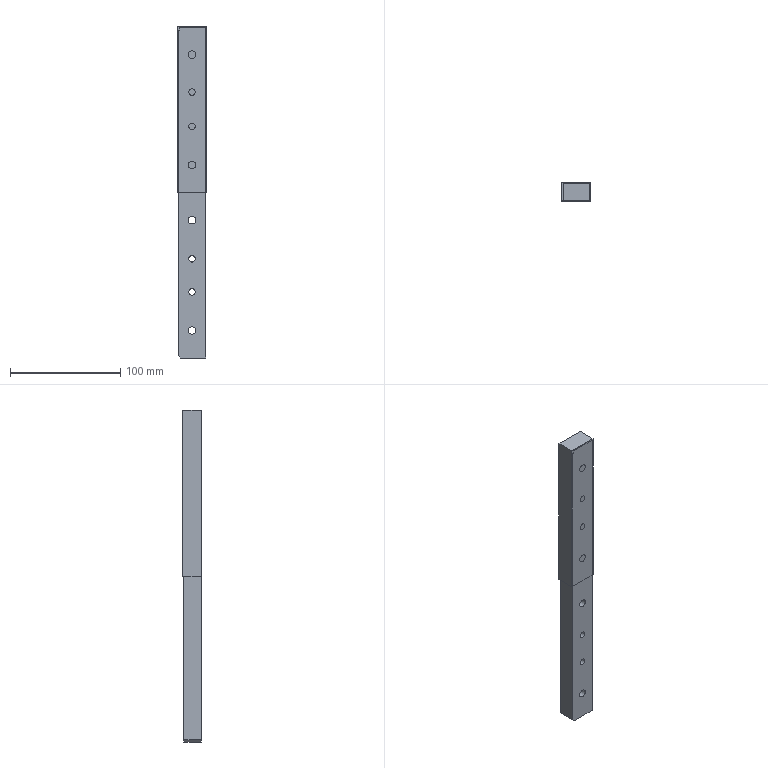Part | NX | features BREP 2 | 2 solids | 39 faces | box 27 x 16.6 x 301 mm | volume 178522 mm3 | plane 23 | cylinder 16 | commonest cylinder face diameters 7 x8 6 x4 11 x4
STEP:
#1=CARTESIAN_POINT('',(12.5,15.6,280.5));
#2=VERTEX_POINT('',#1);
#3=CARTESIAN_POINT('',(12.5,15.6,275.));
#4=DIRECTION('',(0.,1.,0.));
#5=DIRECTION('',(0.,0.,1.));
#6=AXIS2_PLACEMENT_3D('',#3,#4,#5);
#7=CIRCLE('',#6,5.5);
#8=EDGE_CURVE('',#2,#2,#7,.T.);
#9=ORIENTED_EDGE('',*,*,#8,.F.);
#10=EDGE_LOOP('',(#9));
#11=FACE_BOUND('',#10,.T.);
#12=CARTESIAN_POINT('',(12.5,15.6,213.5));
#13=VERTEX_POINT('',#12);
#14=CARTESIAN_POINT('',(12.5,15.6,210.));
#15=DIRECTION('',(0.,1.,0.));
#16=DIRECTION('',(0.,0.,1.));
#17=AXIS2_PLACEMENT_3D('',#14,#15,#16);
#18=CIRCLE('',#17,3.5);
#19=EDGE_CURVE('',#13,#13,#18,.T.);
#20=ORIENTED_EDGE('',*,*,#19,.F.);
#21=EDGE_LOOP('',(#20));
#22=FACE_BOUND('',#21,.T.);
#23=CARTESIAN_POINT('',(12.5,15.6,244.5));
#24=VERTEX_POINT('',#23);
#25=CARTESIAN_POINT('',(12.5,15.6,241.));
#26=DIRECTION('',(0.,1.,0.));
#27=DIRECTION('',(0.,0.,1.));
#28=AXIS2_PLACEMENT_3D('',#25,#26,#27);
#29=CIRCLE('',#28,3.5);
#30=EDGE_CURVE('',#24,#24,#29,.T.);
#31=ORIENTED_EDGE('',*,*,#30,.F.);
#32=EDGE_LOOP('',(#31));
#33=FACE_BOUND('',#32,.T.);
#34=CARTESIAN_POINT('',(12.5,15.6,180.5));
#35=VERTEX_POINT('',#34);
#36=CARTESIAN_POINT('',(12.5,15.6,175.));
#37=DIRECTION('',(0.,1.,0.));
#38=DIRECTION('',(0.,0.,1.));
#39=AXIS2_PLACEMENT_3D('',#36,#37,#38);
#40=CIRCLE('',#39,5.5);
#41=EDGE_CURVE('',#35,#35,#40,.T.);
#42=ORIENTED_EDGE('',*,*,#41,.F.);
#43=EDGE_LOOP('',(#42));
#44=FACE_BOUND('',#43,.T.);
#45=CARTESIAN_POINT('',(12.5,15.6,63.5));
#46=VERTEX_POINT('',#45);
#47=CARTESIAN_POINT('',(12.5,15.6,60.));
#48=DIRECTION('',(0.,1.,0.));
#49=DIRECTION('',(0.,0.,1.));
#50=AXIS2_PLACEMENT_3D('',#47,#48,#49);
#51=CIRCLE('',#50,3.5);
#52=EDGE_CURVE('',#46,#46,#51,.T.);
#53=ORIENTED_EDGE('',*,*,#52,.F.);
#54=EDGE_LOOP('',(#53));
#55=FACE_BOUND('',#54,.T.);
#56=CARTESIAN_POINT('',(12.5,15.6,93.5));
#57=VERTEX_POINT('',#56);
#58=CARTESIAN_POINT('',(12.5,15.6,90.));
#59=DIRECTION('',(0.,1.,0.));
#60=DIRECTION('',(0.,0.,1.));
#61=AXIS2_PLACEMENT_3D('',#58,#59,#60);
#62=CIRCLE('',#61,3.5);
#63=EDGE_CURVE('',#57,#57,#62,.T.);
#64=ORIENTED_EDGE('',*,*,#63,.F.);
#65=EDGE_LOOP('',(#64));
#66=FACE_BOUND('',#65,.T.);
#67=CARTESIAN_POINT('',(12.5,15.6,30.5));
#68=VERTEX_POINT('',#67);
#69=CARTESIAN_POINT('',(12.5,15.6,25.));
#70=DIRECTION('',(0.,1.,0.));
#71=DIRECTION('',(0.,0.,1.));
#72=AXIS2_PLACEMENT_3D('',#69,#70,#71);
#73=CIRCLE('',#72,5.5);
#74=EDGE_CURVE('',#68,#68,#73,.T.);
#75=ORIENTED_EDGE('',*,*,#74,.F.);
#76=EDGE_LOOP('',(#75));
#77=FACE_BOUND('',#76,.T.);
#78=CARTESIAN_POINT('',(12.5,15.6,130.5));
#79=VERTEX_POINT('',#78);
#80=CARTESIAN_POINT('',(12.5,15.6,125.));
#81=DIRECTION('',(0.,1.,0.));
#82=DIRECTION('',(0.,0.,1.));
#83=AXIS2_PLACEMENT_3D('',#80,#81,#82);
#84=CIRCLE('',#83,5.5);
#85=EDGE_CURVE('',#79,#79,#84,.T.);
#86=ORIENTED_EDGE('',*,*,#85,.F.);
#87=EDGE_LOOP('',(#86));
#88=FACE_BOUND('',#87,.T.);
#89=CARTESIAN_POINT('',(0.,15.6,297.342));
#90=VERTEX_POINT('',#89);
#91=CARTESIAN_POINT('',(0.,15.6,2.));
#92=VERTEX_POINT('',#91);
#93=CARTESIAN_POINT('',(0.,15.6,300.));
#94=DIRECTION('',(0.,0.,-1.));
#95=VECTOR('',#94,1000.);
#96=LINE('',#93,#95);
#97=EDGE_CURVE('',#90,#92,#96,.T.);
#98=ORIENTED_EDGE('',*,*,#97,.F.);
#99=CARTESIAN_POINT('',(0.9,15.6,297.342));
#100=VERTEX_POINT('',#99);
#101=CARTESIAN_POINT('',(0.,15.6,297.342));
#102=DIRECTION('',(1.,0.,0.));
#103=VECTOR('',#102,1000.);
#104=LINE('',#101,#103);
#105=EDGE_CURVE('',#90,#100,#104,.T.);
#106=ORIENTED_EDGE('',*,*,#105,.T.);
#107=CARTESIAN_POINT('',(0.9,15.6,300.));
#108=VERTEX_POINT('',#107);
#109=CARTESIAN_POINT('',(0.9,15.6,300.));
#110=DIRECTION('',(0.,0.,1.));
#111=VECTOR('',#110,1000.);
#112=LINE('',#109,#111);
#113=EDGE_CURVE('',#100,#108,#112,.T.);
#114=ORIENTED_EDGE('',*,*,#113,.T.);
#115=CARTESIAN_POINT('',(25.,15.6,300.));
#116=VERTEX_POINT('',#115);
#117=CARTESIAN_POINT('',(0.,15.6,300.));
#118=DIRECTION('',(1.,0.,0.));
#119=VECTOR('',#118,1000.);
#120=LINE('',#117,#119);
#121=EDGE_CURVE('',#108,#116,#120,.T.);
#122=ORIENTED_EDGE('',*,*,#121,.T.);
#123=CARTESIAN_POINT('',(25.,15.6,0.));
#124=VERTEX_POINT('',#123);
#125=CARTESIAN_POINT('',(25.,15.6,300.));
#126=DIRECTION('',(0.,0.,-1.));
#127=VECTOR('',#126,1000.);
#128=LINE('',#125,#127);
#129=EDGE_CURVE('',#116,#124,#128,.T.);
#130=ORIENTED_EDGE('',*,*,#129,.T.);
#131=CARTESIAN_POINT('',(2.,15.6,0.));
#132=VERTEX_POINT('',#131);
#133=CARTESIAN_POINT('',(0.,15.6,0.));
#134=DIRECTION('',(1.,0.,0.));
#135=VECTOR('',#134,1000.);
#136=LINE('',#133,#135);
#137=EDGE_CURVE('',#132,#124,#136,.T.);
#138=ORIENTED_EDGE('',*,*,#137,.F.);
#139=CARTESIAN_POINT('',(-149.,15.6,151.));
#140=DIRECTION('',(-0.7071,0.,0.7071));
#141=VECTOR('',#140,1000.);
#142=LINE('',#139,#141);
#143=EDGE_CURVE('',#132,#92,#142,.T.);
#144=ORIENTED_EDGE('',*,*,#143,.T.);
#145=EDGE_LOOP('',(#98,#106,#114,#122,#130,#138,#144));
#146=FACE_BOUND('',#145,.T.);
#147=CARTESIAN_POINT('',(0.,15.6,300.));
#148=DIRECTION('',(0.,1.,0.));
#149=DIRECTION('',(0.,0.,-1.));
#150=AXIS2_PLACEMENT_3D('',#147,#148,#149);
#151=PLANE('',#150);
#152=ADVANCED_FACE('',(#11,#22,#33,#44,#55,#66,#77,#88,#146),#151,.T.);
#153=CARTESIAN_POINT('',(0.,0.,297.342));
#154=VERTEX_POINT('',#153);
#155=CARTESIAN_POINT('',(0.,0.,2.));
#156=VERTEX_POINT('',#155);
#157=CARTESIAN_POINT('',(0.,0.,300.));
#158=DIRECTION('',(0.,0.,-1.));
#159=VECTOR('',#158,1000.);
#160=LINE('',#157,#159);
#161=EDGE_CURVE('',#154,#156,#160,.T.);
#162=ORIENTED_EDGE('',*,*,#161,.F.);
#163=CARTESIAN_POINT('',(0.,0.,297.342));
#164=DIRECTION('',(0.,1.,0.));
#165=VECTOR('',#164,1000.);
#166=LINE('',#163,#165);
#167=EDGE_CURVE('',#154,#90,#166,.T.);
#168=ORIENTED_EDGE('',*,*,#167,.T.);
#169=ORIENTED_EDGE('',*,*,#97,.T.);
#170=CARTESIAN_POINT('',(0.,0.,2.));
#171=DIRECTION('',(0.,-1.,0.));
#172=VECTOR('',#171,1000.);
#173=LINE('',#170,#172);
#174=EDGE_CURVE('',#92,#156,#173,.T.);
#175=ORIENTED_EDGE('',*,*,#174,.T.);
#176=EDGE_LOOP('',(#162,#168,#169,#175));
#177=FACE_BOUND('',#176,.T.);
#178=CARTESIAN_POINT('',(0.,0.,300.));
#179=DIRECTION('',(-1.,0.,0.));
#180=DIRECTION('',(0.,0.,-1.));
#181=AXIS2_PLACEMENT_3D('',#178,#179,#180);
#182=PLANE('',#181);
#183=ADVANCED_FACE('',(#177),#182,.T.);
#184=CARTESIAN_POINT('',(12.5,0.,271.5));
#185=VERTEX_POINT('',#184);
#186=CARTESIAN_POINT('',(12.5,0.,275.));
#187=DIRECTION('',(0.,-1.,0.));
#188=DIRECTION('',(0.,0.,-1.));
#189=AXIS2_PLACEMENT_3D('',#186,#187,#188);
#190=CIRCLE('',#189,3.5);
#191=EDGE_CURVE('',#185,#185,#190,.T.);
#192=ORIENTED_EDGE('',*,*,#191,.F.);
#193=EDGE_LOOP('',(#192));
#194=FACE_BOUND('',#193,.T.);
#195=CARTESIAN_POINT('',(15.5,0.,210.));
#196=VERTEX_POINT('',#195);
#197=CARTESIAN_POINT('',(12.5,0.,210.));
#198=DIRECTION('',(0.,-1.,0.));
#199=DIRECTION('',(1.,0.,0.));
#200=AXIS2_PLACEMENT_3D('',#197,#198,#199);
#201=CIRCLE('',#200,3.);
#202=EDGE_CURVE('',#196,#196,#201,.T.);
#203=ORIENTED_EDGE('',*,*,#202,.F.);
#204=EDGE_LOOP('',(#203));
#205=FACE_BOUND('',#204,.T.);
#206=CARTESIAN_POINT('',(15.5,0.,241.));
#207=VERTEX_POINT('',#206);
#208=CARTESIAN_POINT('',(12.5,0.,241.));
#209=DIRECTION('',(0.,-1.,0.));
#210=DIRECTION('',(1.,0.,0.));
#211=AXIS2_PLACEMENT_3D('',#208,#209,#210);
#212=CIRCLE('',#211,3.);
#213=EDGE_CURVE('',#207,#207,#212,.T.);
#214=ORIENTED_EDGE('',*,*,#213,.F.);
#215=EDGE_LOOP('',(#214));
#216=FACE_BOUND('',#215,.T.);
#217=CARTESIAN_POINT('',(12.5,0.,171.5));
#218=VERTEX_POINT('',#217);
#219=CARTESIAN_POINT('',(12.5,0.,175.));
#220=DIRECTION('',(0.,-1.,0.));
#221=DIRECTION('',(0.,0.,-1.));
#222=AXIS2_PLACEMENT_3D('',#219,#220,#221);
#223=CIRCLE('',#222,3.5);
#224=EDGE_CURVE('',#218,#218,#223,.T.);
#225=ORIENTED_EDGE('',*,*,#224,.F.);
#226=EDGE_LOOP('',(#225));
#227=FACE_BOUND('',#226,.T.);
#228=CARTESIAN_POINT('',(15.5,0.,60.));
#229=VERTEX_POINT('',#228);
#230=CARTESIAN_POINT('',(12.5,0.,60.));
#231=DIRECTION('',(0.,-1.,0.));
#232=DIRECTION('',(1.,0.,0.));
#233=AXIS2_PLACEMENT_3D('',#230,#231,#232);
#234=CIRCLE('',#233,3.);
#235=EDGE_CURVE('',#229,#229,#234,.T.);
#236=ORIENTED_EDGE('',*,*,#235,.F.);
#237=EDGE_LOOP('',(#236));
#238=FACE_BOUND('',#237,.T.);
#239=CARTESIAN_POINT('',(15.5,0.,90.));
#240=VERTEX_POINT('',#239);
#241=CARTESIAN_POINT('',(12.5,0.,90.));
#242=DIRECTION('',(0.,-1.,0.));
#243=DIRECTION('',(1.,0.,0.));
#244=AXIS2_PLACEMENT_3D('',#241,#242,#243);
#245=CIRCLE('',#244,3.);
#246=EDGE_CURVE('',#240,#240,#245,.T.);
#247=ORIENTED_EDGE('',*,*,#246,.F.);
#248=EDGE_LOOP('',(#247));
#249=FACE_BOUND('',#248,.T.);
#250=CARTESIAN_POINT('',(12.5,0.,21.5));
#251=VERTEX_POINT('',#250);
#252=CARTESIAN_POINT('',(12.5,0.,25.));
#253=DIRECTION('',(0.,-1.,0.));
#254=DIRECTION('',(0.,0.,-1.));
#255=AXIS2_PLACEMENT_3D('',#252,#253,#254);
#256=CIRCLE('',#255,3.5);
#257=EDGE_CURVE('',#251,#251,#256,.T.);
#258=ORIENTED_EDGE('',*,*,#257,.F.);
#259=EDGE_LOOP('',(#258));
#260=FACE_BOUND('',#259,.T.);
#261=CARTESIAN_POINT('',(12.5,0.,121.5));
#262=VERTEX_POINT('',#261);
#263=CARTESIAN_POINT('',(12.5,0.,125.));
#264=DIRECTION('',(0.,-1.,0.));
#265=DIRECTION('',(0.,0.,-1.));
#266=AXIS2_PLACEMENT_3D('',#263,#264,#265);
#267=CIRCLE('',#266,3.5);
#268=EDGE_CURVE('',#262,#262,#267,.T.);
#269=ORIENTED_EDGE('',*,*,#268,.F.);
#270=EDGE_LOOP('',(#269));
#271=FACE_BOUND('',#270,.T.);
#272=CARTESIAN_POINT('',(0.9,0.,300.));
#273=VERTEX_POINT('',#272);
#274=CARTESIAN_POINT('',(0.9,0.,297.342));
#275=VERTEX_POINT('',#274);
#276=CARTESIAN_POINT('',(0.9,0.,300.));
#277=DIRECTION('',(0.,0.,-1.));
#278=VECTOR('',#277,1000.);
#279=LINE('',#276,#278);
#280=EDGE_CURVE('',#273,#275,#279,.T.);
#281=ORIENTED_EDGE('',*,*,#280,.T.);
#282=CARTESIAN_POINT('',(25.,0.,297.342));
#283=DIRECTION('',(-1.,0.,0.));
#284=VECTOR('',#283,1000.);
#285=LINE('',#282,#284);
#286=EDGE_CURVE('',#275,#154,#285,.T.);
#287=ORIENTED_EDGE('',*,*,#286,.T.);
#288=ORIENTED_EDGE('',*,*,#161,.T.);
#289=CARTESIAN_POINT('',(2.,0.,0.));
#290=VERTEX_POINT('',#289);
#291=CARTESIAN_POINT('',(-136.5,0.,138.5));
#292=DIRECTION('',(0.7071,0.,-0.7071));
#293=VECTOR('',#292,1000.);
#294=LINE('',#291,#293);
#295=EDGE_CURVE('',#156,#290,#294,.T.);
#296=ORIENTED_EDGE('',*,*,#295,.T.);
#297=CARTESIAN_POINT('',(25.,0.,0.));
#298=VERTEX_POINT('',#297);
#299=CARTESIAN_POINT('',(25.,0.,0.));
#300=DIRECTION('',(-1.,0.,0.));
#301=VECTOR('',#300,1000.);
#302=LINE('',#299,#301);
#303=EDGE_CURVE('',#298,#290,#302,.T.);
#304=ORIENTED_EDGE('',*,*,#303,.F.);
#305=CARTESIAN_POINT('',(25.,0.,300.));
#306=VERTEX_POINT('',#305);
#307=CARTESIAN_POINT('',(25.,0.,300.));
#308=DIRECTION('',(0.,0.,-1.));
#309=VECTOR('',#308,1000.);
#310=LINE('',#307,#309);
#311=EDGE_CURVE('',#306,#298,#310,.T.);
#312=ORIENTED_EDGE('',*,*,#311,.F.);
#313=CARTESIAN_POINT('',(25.,0.,300.));
#314=DIRECTION('',(-1.,0.,0.));
#315=VECTOR('',#314,1000.);
#316=LINE('',#313,#315);
#317=EDGE_CURVE('',#306,#273,#316,.T.);
#318=ORIENTED_EDGE('',*,*,#317,.T.);
#319=EDGE_LOOP('',(#281,#287,#288,#296,#304,#312,#318));
#320=FACE_BOUND('',#319,.T.);
#321=CARTESIAN_POINT('',(25.,0.,300.));
#322=DIRECTION('',(0.,-1.,0.));
#323=DIRECTION('',(-1.,0.,0.));
#324=AXIS2_PLACEMENT_3D('',#321,#322,#323);
#325=PLANE('',#324);
#326=ADVANCED_FACE('',(#194,#205,#216,#227,#238,#249,#260,#271,#320),#325,.T.);
#327=CARTESIAN_POINT('',(0.9,0.,300.));
#328=DIRECTION('',(0.,1.,0.));
#329=VECTOR('',#328,1000.);
#330=LINE('',#327,#329);
#331=EDGE_CURVE('',#273,#108,#330,.T.);
#332=ORIENTED_EDGE('',*,*,#331,.F.);
#333=ORIENTED_EDGE('',*,*,#317,.F.);
#334=CARTESIAN_POINT('',(25.,15.6,300.));
#335=DIRECTION('',(0.,-1.,0.));
#336=VECTOR('',#335,1000.);
#337=LINE('',#334,#336);
#338=EDGE_CURVE('',#116,#306,#337,.T.);
#339=ORIENTED_EDGE('',*,*,#338,.F.);
#340=ORIENTED_EDGE('',*,*,#121,.F.);
#341=EDGE_LOOP('',(#332,#333,#339,#340));
#342=FACE_BOUND('',#341,.T.);
#343=CARTESIAN_POINT('',(25.,0.,300.));
#344=DIRECTION('',(0.,0.,-1.));
#345=DIRECTION('',(1.,0.,0.));
#346=AXIS2_PLACEMENT_3D('',#343,#344,#345);
#347=PLANE('',#346);
#348=ADVANCED_FACE('',(#342),#347,.F.);
#349=ORIENTED_EDGE('',*,*,#311,.T.);
#350=CARTESIAN_POINT('',(25.,15.6,0.));
#351=DIRECTION('',(0.,-1.,0.));
#352=VECTOR('',#351,1000.);
#353=LINE('',#350,#352);
#354=EDGE_CURVE('',#124,#298,#353,.T.);
#355=ORIENTED_EDGE('',*,*,#354,.F.);
#356=ORIENTED_EDGE('',*,*,#129,.F.);
#357=ORIENTED_EDGE('',*,*,#338,.T.);
#358=EDGE_LOOP('',(#349,#355,#356,#357));
#359=FACE_BOUND('',#358,.T.);
#360=CARTESIAN_POINT('',(25.,15.6,300.));
#361=DIRECTION('',(1.,0.,0.));
#362=DIRECTION('',(0.,-1.,0.));
#363=AXIS2_PLACEMENT_3D('',#360,#361,#362);
#364=PLANE('',#363);
#365=ADVANCED_FACE('',(#359),#364,.T.);
#366=ORIENTED_EDGE('',*,*,#303,.T.);
#367=CARTESIAN_POINT('',(2.,0.,0.));
#368=DIRECTION('',(0.,1.,0.));
#369=VECTOR('',#368,1000.);
#370=LINE('',#367,#369);
#371=EDGE_CURVE('',#290,#132,#370,.T.);
#372=ORIENTED_EDGE('',*,*,#371,.T.);
#373=ORIENTED_EDGE('',*,*,#137,.T.);
#374=ORIENTED_EDGE('',*,*,#354,.T.);
#375=EDGE_LOOP('',(#366,#372,#373,#374));
#376=FACE_BOUND('',#375,.T.);
#377=CARTESIAN_POINT('',(25.,0.,0.));
#378=DIRECTION('',(0.,0.,-1.));
#379=DIRECTION('',(1.,0.,0.));
#380=AXIS2_PLACEMENT_3D('',#377,#378,#379);
#381=PLANE('',#380);
#382=ADVANCED_FACE('',(#376),#381,.T.);
#383=ORIENTED_EDGE('',*,*,#295,.F.);
#384=ORIENTED_EDGE('',*,*,#174,.F.);
#385=ORIENTED_EDGE('',*,*,#143,.F.);
#386=ORIENTED_EDGE('',*,*,#371,.F.);
#387=EDGE_LOOP('',(#383,#384,#385,#386));
#388=FACE_BOUND('',#387,.T.);
#389=CARTESIAN_POINT('',(2.,0.,0.));
#390=DIRECTION('',(0.7071,0.,0.7071));
#391=DIRECTION('',(-0.7071,0.,0.7071));
#392=AXIS2_PLACEMENT_3D('',#389,#390,#391);
#393=PLANE('',#392);
#394=ADVANCED_FACE('',(#388),#393,.F.);
#395=ORIENTED_EDGE('',*,*,#167,.F.);
#396=ORIENTED_EDGE('',*,*,#286,.F.);
#397=CARTESIAN_POINT('',(0.9,0.6,297.342));
#398=DIRECTION('',(0.,-1.,0.));
#399=VECTOR('',#398,1000.);
#400=LINE('',#397,#399);
#401=EDGE_CURVE('',#100,#275,#400,.T.);
#402=ORIENTED_EDGE('',*,*,#401,.F.);
#403=ORIENTED_EDGE('',*,*,#105,.F.);
#404=EDGE_LOOP('',(#395,#396,#402,#403));
#405=FACE_BOUND('',#404,.T.);
#406=CARTESIAN_POINT('',(-30.1,0.6,297.342));
#407=DIRECTION('',(0.,0.,1.));
#408=DIRECTION('',(-1.,0.,0.));
#409=AXIS2_PLACEMENT_3D('',#406,#407,#408);
#410=PLANE('',#409);
#411=ADVANCED_FACE('',(#405),#410,.T.);
#412=ORIENTED_EDGE('',*,*,#401,.T.);
#413=ORIENTED_EDGE('',*,*,#280,.F.);
#414=ORIENTED_EDGE('',*,*,#331,.T.);
#415=ORIENTED_EDGE('',*,*,#113,.F.);
#416=EDGE_LOOP('',(#412,#413,#414,#415));
#417=FACE_BOUND('',#416,.T.);
#418=CARTESIAN_POINT('',(0.9,0.6,277.75));
#419=DIRECTION('',(-1.,0.,0.));
#420=DIRECTION('',(0.,0.,-1.));
#421=AXIS2_PLACEMENT_3D('',#418,#419,#420);
#422=PLANE('',#421);
#423=ADVANCED_FACE('',(#417),#422,.T.);
#424=ORIENTED_EDGE('',*,*,#268,.T.);
#425=EDGE_LOOP('',(#424));
#426=FACE_BOUND('',#425,.T.);
#427=CARTESIAN_POINT('',(12.5,7.6,121.5));
#428=VERTEX_POINT('',#427);
#429=CARTESIAN_POINT('',(12.5,7.6,125.));
#430=DIRECTION('',(0.,1.,0.));
#431=DIRECTION('',(0.,0.,-1.));
#432=AXIS2_PLACEMENT_3D('',#429,#430,#431);
#433=CIRCLE('',#432,3.5);
#434=EDGE_CURVE('',#428,#428,#433,.T.);
#435=ORIENTED_EDGE('',*,*,#434,.T.);
#436=EDGE_LOOP('',(#435));
#437=FACE_BOUND('',#436,.T.);
#438=CARTESIAN_POINT('',(12.5,7.6,125.));
#439=DIRECTION('',(0.,-1.,0.));
#440=DIRECTION('',(0.,0.,1.));
#441=AXIS2_PLACEMENT_3D('',#438,#439,#440);
#442=CYLINDRICAL_SURFACE('',#441,3.5);
#443=ADVANCED_FACE('',(#426,#437),#442,.F.);
#444=ORIENTED_EDGE('',*,*,#85,.T.);
#445=EDGE_LOOP('',(#444));
#446=FACE_BOUND('',#445,.T.);
#447=CARTESIAN_POINT('',(12.5,7.6,130.5));
#448=VERTEX_POINT('',#447);
#449=CARTESIAN_POINT('',(12.5,7.6,125.));
#450=DIRECTION('',(0.,-1.,0.));
#451=DIRECTION('',(0.,0.,1.));
#452=AXIS2_PLACEMENT_3D('',#449,#450,#451);
#453=CIRCLE('',#452,5.5);
#454=EDGE_CURVE('',#448,#448,#453,.T.);
#455=ORIENTED_EDGE('',*,*,#454,.T.);
#456=EDGE_LOOP('',(#455));
#457=FACE_BOUND('',#456,.T.);
#458=CARTESIAN_POINT('',(12.5,7.6,125.));
#459=DIRECTION('',(0.,1.,0.));
#460=DIRECTION('',(0.,0.,-1.));
#461=AXIS2_PLACEMENT_3D('',#458,#459,#460);
#462=CYLINDRICAL_SURFACE('',#461,5.5);
#463=ADVANCED_FACE('',(#446,#457),#462,.F.);
#464=ORIENTED_EDGE('',*,*,#434,.F.);
#465=EDGE_LOOP('',(#464));
#466=FACE_BOUND('',#465,.T.);
#467=ORIENTED_EDGE('',*,*,#454,.F.);
#468=EDGE_LOOP('',(#467));
#469=FACE_BOUND('',#468,.T.);
#470=CARTESIAN_POINT('',(12.5,7.6,125.));
#471=DIRECTION('',(0.,-1.,0.));
#472=DIRECTION('',(0.,0.,1.));
#473=AXIS2_PLACEMENT_3D('',#470,#471,#472);
#474=PLANE('',#473);
#475=ADVANCED_FACE('',(#466,#469),#474,.F.);
#476=ORIENTED_EDGE('',*,*,#257,.T.);
#477=EDGE_LOOP('',(#476));
#478=FACE_BOUND('',#477,.T.);
#479=CARTESIAN_POINT('',(12.5,7.6,21.5));
#480=VERTEX_POINT('',#479);
#481=CARTESIAN_POINT('',(12.5,7.6,25.));
#482=DIRECTION('',(0.,1.,0.));
#483=DIRECTION('',(0.,0.,-1.));
#484=AXIS2_PLACEMENT_3D('',#481,#482,#483);
#485=CIRCLE('',#484,3.5);
#486=EDGE_CURVE('',#480,#480,#485,.T.);
#487=ORIENTED_EDGE('',*,*,#486,.T.);
#488=EDGE_LOOP('',(#487));
#489=FACE_BOUND('',#488,.T.);
#490=CARTESIAN_POINT('',(12.5,7.6,25.));
#491=DIRECTION('',(0.,-1.,0.));
#492=DIRECTION('',(0.,0.,1.));
#493=AXIS2_PLACEMENT_3D('',#490,#491,#492);
#494=CYLINDRICAL_SURFACE('',#493,3.5);
#495=ADVANCED_FACE('',(#478,#489),#494,.F.);
#496=ORIENTED_EDGE('',*,*,#74,.T.);
#497=EDGE_LOOP('',(#496));
#498=FACE_BOUND('',#497,.T.);
#499=CARTESIAN_POINT('',(12.5,7.6,30.5));
#500=VERTEX_POINT('',#499);
#501=CARTESIAN_POINT('',(12.5,7.6,25.));
#502=DIRECTION('',(0.,-1.,0.));
#503=DIRECTION('',(0.,0.,1.));
#504=AXIS2_PLACEMENT_3D('',#501,#502,#503);
#505=CIRCLE('',#504,5.5);
#506=EDGE_CURVE('',#500,#500,#505,.T.);
#507=ORIENTED_EDGE('',*,*,#506,.T.);
#508=EDGE_LOOP('',(#507));
#509=FACE_BOUND('',#508,.T.);
#510=CARTESIAN_POINT('',(12.5,7.6,25.));
#511=DIRECTION('',(0.,1.,0.));
#512=DIRECTION('',(0.,0.,-1.));
#513=AXIS2_PLACEMENT_3D('',#510,#511,#512);
#514=CYLINDRICAL_SURFACE('',#513,5.5);
#515=ADVANCED_FACE('',(#498,#509),#514,.F.);
#516=ORIENTED_EDGE('',*,*,#486,.F.);
#517=EDGE_LOOP('',(#516));
#518=FACE_BOUND('',#517,.T.);
#519=ORIENTED_EDGE('',*,*,#506,.F.);
#520=EDGE_LOOP('',(#519));
#521=FACE_BOUND('',#520,.T.);
#522=CARTESIAN_POINT('',(12.5,7.6,25.));
#523=DIRECTION('',(0.,-1.,0.));
#524=DIRECTION('',(0.,0.,1.));
#525=AXIS2_PLACEMENT_3D('',#522,#523,#524);
#526=PLANE('',#525);
#527=ADVANCED_FACE('',(#518,#521),#526,.F.);
#528=CARTESIAN_POINT('',(12.5,13.1,93.5));
#529=VERTEX_POINT('',#528);
#530=CARTESIAN_POINT('',(12.5,13.1,90.));
#531=DIRECTION('',(0.,-1.,0.));
#532=DIRECTION('',(0.,0.,1.));
#533=AXIS2_PLACEMENT_3D('',#530,#531,#532);
#534=CIRCLE('',#533,3.5);
#535=EDGE_CURVE('',#529,#529,#534,.T.);
#536=ORIENTED_EDGE('',*,*,#535,.T.);
#537=EDGE_LOOP('',(#536));
#538=FACE_BOUND('',#537,.T.);
#539=ORIENTED_EDGE('',*,*,#63,.T.);
#540=EDGE_LOOP('',(#539));
#541=FACE_BOUND('',#540,.T.);
#542=CARTESIAN_POINT('',(12.5,13.1,90.));
#543=DIRECTION('',(0.,1.,0.));
#544=DIRECTION('',(0.,0.,-1.));
#545=AXIS2_PLACEMENT_3D('',#542,#543,#544);
#546=CYLINDRICAL_SURFACE('',#545,3.5);
#547=ADVANCED_FACE('',(#538,#541),#546,.F.);
#548=CARTESIAN_POINT('',(12.5,13.1,87.));
#549=VERTEX_POINT('',#548);
#550=CARTESIAN_POINT('',(12.5,13.1,90.));
#551=DIRECTION('',(0.,1.,0.));
#552=DIRECTION('',(0.,0.,-1.));
#553=AXIS2_PLACEMENT_3D('',#550,#551,#552);
#554=CIRCLE('',#553,3.);
#555=EDGE_CURVE('',#549,#549,#554,.T.);
#556=ORIENTED_EDGE('',*,*,#555,.F.);
#557=EDGE_LOOP('',(#556));
#558=FACE_BOUND('',#557,.T.);
#559=ORIENTED_EDGE('',*,*,#535,.F.);
#560=EDGE_LOOP('',(#559));
#561=FACE_BOUND('',#560,.T.);
#562=CARTESIAN_POINT('',(12.5,13.1,90.));
#563=DIRECTION('',(0.,1.,0.));
#564=DIRECTION('',(0.,0.,-1.));
#565=AXIS2_PLACEMENT_3D('',#562,#563,#564);
#566=PLANE('',#565);
#567=ADVANCED_FACE('',(#558,#561),#566,.T.);
#568=ORIENTED_EDGE('',*,*,#246,.T.);
#569=EDGE_LOOP('',(#568));
#570=FACE_BOUND('',#569,.T.);
#571=ORIENTED_EDGE('',*,*,#555,.T.);
#572=EDGE_LOOP('',(#571));
#573=FACE_BOUND('',#572,.T.);
#574=CARTESIAN_POINT('',(12.5,13.1,90.));
#575=DIRECTION('',(0.,-1.,0.));
#576=DIRECTION('',(0.,0.,1.));
#577=AXIS2_PLACEMENT_3D('',#574,#575,#576);
#578=CYLINDRICAL_SURFACE('',#577,3.);
#579=ADVANCED_FACE('',(#570,#573),#578,.F.);
#580=CARTESIAN_POINT('',(12.5,13.1,63.5));
#581=VERTEX_POINT('',#580);
#582=CARTESIAN_POINT('',(12.5,13.1,60.));
#583=DIRECTION('',(0.,-1.,0.));
#584=DIRECTION('',(0.,0.,1.));
#585=AXIS2_PLACEMENT_3D('',#582,#583,#584);
#586=CIRCLE('',#585,3.5);
#587=EDGE_CURVE('',#581,#581,#586,.T.);
#588=ORIENTED_EDGE('',*,*,#587,.T.);
#589=EDGE_LOOP('',(#588));
#590=FACE_BOUND('',#589,.T.);
#591=ORIENTED_EDGE('',*,*,#52,.T.);
#592=EDGE_LOOP('',(#591));
#593=FACE_BOUND('',#592,.T.);
#594=CARTESIAN_POINT('',(12.5,13.1,60.));
#595=DIRECTION('',(0.,1.,0.));
#596=DIRECTION('',(0.,0.,-1.));
#597=AXIS2_PLACEMENT_3D('',#594,#595,#596);
#598=CYLINDRICAL_SURFACE('',#597,3.5);
#599=ADVANCED_FACE('',(#590,#593),#598,.F.);
#600=CARTESIAN_POINT('',(12.5,13.1,57.));
#601=VERTEX_POINT('',#600);
#602=CARTESIAN_POINT('',(12.5,13.1,60.));
#603=DIRECTION('',(0.,1.,0.));
#604=DIRECTION('',(0.,0.,-1.));
#605=AXIS2_PLACEMENT_3D('',#602,#603,#604);
#606=CIRCLE('',#605,3.);
#607=EDGE_CURVE('',#601,#601,#606,.T.);
#608=ORIENTED_EDGE('',*,*,#607,.F.);
#609=EDGE_LOOP('',(#608));
#610=FACE_BOUND('',#609,.T.);
#611=ORIENTED_EDGE('',*,*,#587,.F.);
#612=EDGE_LOOP('',(#611));
#613=FACE_BOUND('',#612,.T.);
#614=CARTESIAN_POINT('',(12.5,13.1,60.));
#615=DIRECTION('',(0.,1.,0.));
#616=DIRECTION('',(0.,0.,-1.));
#617=AXIS2_PLACEMENT_3D('',#614,#615,#616);
#618=PLANE('',#617);
#619=ADVANCED_FACE('',(#610,#613),#618,.T.);
#620=ORIENTED_EDGE('',*,*,#235,.T.);
#621=EDGE_LOOP('',(#620));
#622=FACE_BOUND('',#621,.T.);
#623=ORIENTED_EDGE('',*,*,#607,.T.);
#624=EDGE_LOOP('',(#623));
#625=FACE_BOUND('',#624,.T.);
#626=CARTESIAN_POINT('',(12.5,13.1,60.));
#627=DIRECTION('',(0.,-1.,0.));
#628=DIRECTION('',(0.,0.,1.));
#629=AXIS2_PLACEMENT_3D('',#626,#627,#628);
#630=CYLINDRICAL_SURFACE('',#629,3.);
#631=ADVANCED_FACE('',(#622,#625),#630,.F.);
#632=ORIENTED_EDGE('',*,*,#224,.T.);
#633=EDGE_LOOP('',(#632));
#634=FACE_BOUND('',#633,.T.);
#635=CARTESIAN_POINT('',(12.5,7.6,171.5));
#636=VERTEX_POINT('',#635);
#637=CARTESIAN_POINT('',(12.5,7.6,175.));
#638=DIRECTION('',(0.,1.,0.));
#639=DIRECTION('',(0.,0.,-1.));
#640=AXIS2_PLACEMENT_3D('',#637,#638,#639);
#641=CIRCLE('',#640,3.5);
#642=EDGE_CURVE('',#636,#636,#641,.T.);
#643=ORIENTED_EDGE('',*,*,#642,.T.);
#644=EDGE_LOOP('',(#643));
#645=FACE_BOUND('',#644,.T.);
#646=CARTESIAN_POINT('',(12.5,7.6,175.));
#647=DIRECTION('',(0.,-1.,0.));
#648=DIRECTION('',(0.,0.,1.));
#649=AXIS2_PLACEMENT_3D('',#646,#647,#648);
#650=CYLINDRICAL_SURFACE('',#649,3.5);
#651=ADVANCED_FACE('',(#634,#645),#650,.F.);
#652=ORIENTED_EDGE('',*,*,#41,.T.);
#653=EDGE_LOOP('',(#652));
#654=FACE_BOUND('',#653,.T.);
#655=CARTESIAN_POINT('',(12.5,7.6,180.5));
#656=VERTEX_POINT('',#655);
#657=CARTESIAN_POINT('',(12.5,7.6,175.));
#658=DIRECTION('',(0.,-1.,0.));
#659=DIRECTION('',(0.,0.,1.));
#660=AXIS2_PLACEMENT_3D('',#657,#658,#659);
#661=CIRCLE('',#660,5.5);
#662=EDGE_CURVE('',#656,#656,#661,.T.);
#663=ORIENTED_EDGE('',*,*,#662,.T.);
#664=EDGE_LOOP('',(#663));
#665=FACE_BOUND('',#664,.T.);
#666=CARTESIAN_POINT('',(12.5,7.6,175.));
#667=DIRECTION('',(0.,1.,0.));
#668=DIRECTION('',(0.,0.,-1.));
#669=AXIS2_PLACEMENT_3D('',#666,#667,#668);
#670=CYLINDRICAL_SURFACE('',#669,5.5);
#671=ADVANCED_FACE('',(#654,#665),#670,.F.);
#672=ORIENTED_EDGE('',*,*,#642,.F.);
#673=EDGE_LOOP('',(#672));
#674=FACE_BOUND('',#673,.T.);
#675=ORIENTED_EDGE('',*,*,#662,.F.);
#676=EDGE_LOOP('',(#675));
#677=FACE_BOUND('',#676,.T.);
#678=CARTESIAN_POINT('',(12.5,7.6,175.));
#679=DIRECTION('',(0.,-1.,0.));
#680=DIRECTION('',(0.,0.,1.));
#681=AXIS2_PLACEMENT_3D('',#678,#679,#680);
#682=PLANE('',#681);
#683=ADVANCED_FACE('',(#674,#677),#682,.F.);
#684=CARTESIAN_POINT('',(12.5,12.6,244.5));
#685=VERTEX_POINT('',#684);
#686=CARTESIAN_POINT('',(12.5,12.6,241.));
#687=DIRECTION('',(0.,-1.,0.));
#688=DIRECTION('',(0.,0.,1.));
#689=AXIS2_PLACEMENT_3D('',#686,#687,#688);
#690=CIRCLE('',#689,3.5);
#691=EDGE_CURVE('',#685,#685,#690,.T.);
#692=ORIENTED_EDGE('',*,*,#691,.T.);
#693=EDGE_LOOP('',(#692));
#694=FACE_BOUND('',#693,.T.);
#695=ORIENTED_EDGE('',*,*,#30,.T.);
#696=EDGE_LOOP('',(#695));
#697=FACE_BOUND('',#696,.T.);
#698=CARTESIAN_POINT('',(12.5,12.6,241.));
#699=DIRECTION('',(0.,1.,0.));
#700=DIRECTION('',(0.,0.,-1.));
#701=AXIS2_PLACEMENT_3D('',#698,#699,#700);
#702=CYLINDRICAL_SURFACE('',#701,3.5);
#703=ADVANCED_FACE('',(#694,#697),#702,.F.);
#704=CARTESIAN_POINT('',(12.5,12.6,238.));
#705=VERTEX_POINT('',#704);
#706=CARTESIAN_POINT('',(12.5,12.6,241.));
#707=DIRECTION('',(0.,1.,0.));
#708=DIRECTION('',(0.,0.,-1.));
#709=AXIS2_PLACEMENT_3D('',#706,#707,#708);
#710=CIRCLE('',#709,3.);
#711=EDGE_CURVE('',#705,#705,#710,.T.);
#712=ORIENTED_EDGE('',*,*,#711,.F.);
#713=EDGE_LOOP('',(#712));
#714=FACE_BOUND('',#713,.T.);
#715=ORIENTED_EDGE('',*,*,#691,.F.);
#716=EDGE_LOOP('',(#715));
#717=FACE_BOUND('',#716,.T.);
#718=CARTESIAN_POINT('',(12.5,12.6,241.));
#719=DIRECTION('',(0.,1.,0.));
#720=DIRECTION('',(0.,0.,-1.));
#721=AXIS2_PLACEMENT_3D('',#718,#719,#720);
#722=PLANE('',#721);
#723=ADVANCED_FACE('',(#714,#717),#722,.T.);
#724=ORIENTED_EDGE('',*,*,#213,.T.);
#725=EDGE_LOOP('',(#724));
#726=FACE_BOUND('',#725,.T.);
#727=ORIENTED_EDGE('',*,*,#711,.T.);
#728=EDGE_LOOP('',(#727));
#729=FACE_BOUND('',#728,.T.);
#730=CARTESIAN_POINT('',(12.5,12.6,241.));
#731=DIRECTION('',(0.,-1.,0.));
#732=DIRECTION('',(0.,0.,1.));
#733=AXIS2_PLACEMENT_3D('',#730,#731,#732);
#734=CYLINDRICAL_SURFACE('',#733,3.);
#735=ADVANCED_FACE('',(#726,#729),#734,.F.);
#736=CARTESIAN_POINT('',(12.5,12.6,213.5));
#737=VERTEX_POINT('',#736);
#738=CARTESIAN_POINT('',(12.5,12.6,210.));
#739=DIRECTION('',(0.,-1.,0.));
#740=DIRECTION('',(0.,0.,1.));
#741=AXIS2_PLACEMENT_3D('',#738,#739,#740);
#742=CIRCLE('',#741,3.5);
#743=EDGE_CURVE('',#737,#737,#742,.T.);
#744=ORIENTED_EDGE('',*,*,#743,.T.);
#745=EDGE_LOOP('',(#744));
#746=FACE_BOUND('',#745,.T.);
#747=ORIENTED_EDGE('',*,*,#19,.T.);
#748=EDGE_LOOP('',(#747));
#749=FACE_BOUND('',#748,.T.);
#750=CARTESIAN_POINT('',(12.5,12.6,210.));
#751=DIRECTION('',(0.,1.,0.));
#752=DIRECTION('',(0.,0.,-1.));
#753=AXIS2_PLACEMENT_3D('',#750,#751,#752);
#754=CYLINDRICAL_SURFACE('',#753,3.5);
#755=ADVANCED_FACE('',(#746,#749),#754,.F.);
#756=CARTESIAN_POINT('',(12.5,12.6,207.));
#757=VERTEX_POINT('',#756);
#758=CARTESIAN_POINT('',(12.5,12.6,210.));
#759=DIRECTION('',(0.,1.,0.));
#760=DIRECTION('',(0.,0.,-1.));
#761=AXIS2_PLACEMENT_3D('',#758,#759,#760);
#762=CIRCLE('',#761,3.);
#763=EDGE_CURVE('',#757,#757,#762,.T.);
#764=ORIENTED_EDGE('',*,*,#763,.F.);
#765=EDGE_LOOP('',(#764));
#766=FACE_BOUND('',#765,.T.);
#767=ORIENTED_EDGE('',*,*,#743,.F.);
#768=EDGE_LOOP('',(#767));
#769=FACE_BOUND('',#768,.T.);
#770=CARTESIAN_POINT('',(12.5,12.6,210.));
#771=DIRECTION('',(0.,1.,0.));
#772=DIRECTION('',(0.,0.,-1.));
#773=AXIS2_PLACEMENT_3D('',#770,#771,#772);
#774=PLANE('',#773);
#775=ADVANCED_FACE('',(#766,#769),#774,.T.);
#776=ORIENTED_EDGE('',*,*,#202,.T.);
#777=EDGE_LOOP('',(#776));
#778=FACE_BOUND('',#777,.T.);
#779=ORIENTED_EDGE('',*,*,#763,.T.);
#780=EDGE_LOOP('',(#779));
#781=FACE_BOUND('',#780,.T.);
#782=CARTESIAN_POINT('',(12.5,12.6,210.));
#783=DIRECTION('',(0.,-1.,0.));
#784=DIRECTION('',(0.,0.,1.));
#785=AXIS2_PLACEMENT_3D('',#782,#783,#784);
#786=CYLINDRICAL_SURFACE('',#785,3.);
#787=ADVANCED_FACE('',(#778,#781),#786,.F.);
#788=ORIENTED_EDGE('',*,*,#191,.T.);
#789=EDGE_LOOP('',(#788));
#790=FACE_BOUND('',#789,.T.);
#791=CARTESIAN_POINT('',(12.5,7.6,271.5));
#792=VERTEX_POINT('',#791);
#793=CARTESIAN_POINT('',(12.5,7.6,275.));
#794=DIRECTION('',(0.,1.,0.));
#795=DIRECTION('',(0.,0.,-1.));
#796=AXIS2_PLACEMENT_3D('',#793,#794,#795);
#797=CIRCLE('',#796,3.5);
#798=EDGE_CURVE('',#792,#792,#797,.T.);
#799=ORIENTED_EDGE('',*,*,#798,.T.);
#800=EDGE_LOOP('',(#799));
#801=FACE_BOUND('',#800,.T.);
#802=CARTESIAN_POINT('',(12.5,7.6,275.));
#803=DIRECTION('',(0.,-1.,0.));
#804=DIRECTION('',(0.,0.,1.));
#805=AXIS2_PLACEMENT_3D('',#802,#803,#804);
#806=CYLINDRICAL_SURFACE('',#805,3.5);
#807=ADVANCED_FACE('',(#790,#801),#806,.F.);
#808=ORIENTED_EDGE('',*,*,#8,.T.);
#809=EDGE_LOOP('',(#808));
#810=FACE_BOUND('',#809,.T.);
#811=CARTESIAN_POINT('',(12.5,7.6,280.5));
#812=VERTEX_POINT('',#811);
#813=CARTESIAN_POINT('',(12.5,7.6,275.));
#814=DIRECTION('',(0.,-1.,0.));
#815=DIRECTION('',(0.,0.,1.));
#816=AXIS2_PLACEMENT_3D('',#813,#814,#815);
#817=CIRCLE('',#816,5.5);
#818=EDGE_CURVE('',#812,#812,#817,.T.);
#819=ORIENTED_EDGE('',*,*,#818,.T.);
#820=EDGE_LOOP('',(#819));
#821=FACE_BOUND('',#820,.T.);
#822=CARTESIAN_POINT('',(12.5,7.6,275.));
#823=DIRECTION('',(0.,1.,0.));
#824=DIRECTION('',(0.,0.,-1.));
#825=AXIS2_PLACEMENT_3D('',#822,#823,#824);
#826=CYLINDRICAL_SURFACE('',#825,5.5);
#827=ADVANCED_FACE('',(#810,#821),#826,.F.);
#828=ORIENTED_EDGE('',*,*,#798,.F.);
#829=EDGE_LOOP('',(#828));
#830=FACE_BOUND('',#829,.T.);
#831=ORIENTED_EDGE('',*,*,#818,.F.);
#832=EDGE_LOOP('',(#831));
#833=FACE_BOUND('',#832,.T.);
#834=CARTESIAN_POINT('',(12.5,7.6,275.));
#835=DIRECTION('',(0.,-1.,0.));
#836=DIRECTION('',(0.,0.,1.));
#837=AXIS2_PLACEMENT_3D('',#834,#835,#836);
#838=PLANE('',#837);
#839=ADVANCED_FACE('',(#830,#833),#838,.F.);
#840=CLOSED_SHELL('',(#152,#183,#326,#348,#365,#382,#394,#411,#423,#443,#463,#475,#495,#515,#527,#547,#567,#579,#599,#619,#631,#651,#671,#683,#703,#723,#735,#755,#775,#787,#807,#827,#839));
#841=MANIFOLD_SOLID_BREP('',#840);
#842=CARTESIAN_POINT('',(26.,16.6,150.));
#843=VERTEX_POINT('',#842);
#844=CARTESIAN_POINT('',(26.,0.,150.));
#845=VERTEX_POINT('',#844);
#846=CARTESIAN_POINT('',(26.,0.,150.));
#847=DIRECTION('',(0.,-1.,0.));
#848=VECTOR('',#847,1000.);
#849=LINE('',#846,#848);
#850=EDGE_CURVE('',#843,#845,#849,.T.);
#851=ORIENTED_EDGE('',*,*,#850,.F.);
#852=CARTESIAN_POINT('',(26.,16.6,301.));
#853=VERTEX_POINT('',#852);
#854=CARTESIAN_POINT('',(26.,16.6,301.));
#855=DIRECTION('',(0.,0.,-1.));
#856=VECTOR('',#855,1000.);
#857=LINE('',#854,#856);
#858=EDGE_CURVE('',#853,#843,#857,.T.);
#859=ORIENTED_EDGE('',*,*,#858,.F.);
#860=CARTESIAN_POINT('',(26.,0.,301.));
#861=VERTEX_POINT('',#860);
#862=CARTESIAN_POINT('',(26.,0.,301.));
#863=DIRECTION('',(0.,-1.,0.));
#864=VECTOR('',#863,1000.);
#865=LINE('',#862,#864);
#866=EDGE_CURVE('',#853,#861,#865,.T.);
#867=ORIENTED_EDGE('',*,*,#866,.T.);
#868=CARTESIAN_POINT('',(26.,0.,301.));
#869=DIRECTION('',(0.,0.,-1.));
#870=VECTOR('',#869,1000.);
#871=LINE('',#868,#870);
#872=EDGE_CURVE('',#861,#845,#871,.T.);
#873=ORIENTED_EDGE('',*,*,#872,.T.);
#874=EDGE_LOOP('',(#851,#859,#867,#873));
#875=FACE_BOUND('',#874,.T.);
#876=CARTESIAN_POINT('',(26.,15.6,301.));
#877=DIRECTION('',(1.,0.,0.));
#878=DIRECTION('',(0.,-1.,0.));
#879=AXIS2_PLACEMENT_3D('',#876,#877,#878);
#880=PLANE('',#879);
#881=ADVANCED_FACE('',(#875),#880,.T.);
#882=CARTESIAN_POINT('',(-1.,16.6,150.));
#883=VERTEX_POINT('',#882);
#884=CARTESIAN_POINT('',(25.,16.6,150.));
#885=DIRECTION('',(1.,0.,0.));
#886=VECTOR('',#885,1000.);
#887=LINE('',#884,#886);
#888=EDGE_CURVE('',#883,#843,#887,.T.);
#889=ORIENTED_EDGE('',*,*,#888,.F.);
#890=CARTESIAN_POINT('',(-1.,16.6,301.));
#891=VERTEX_POINT('',#890);
#892=CARTESIAN_POINT('',(-1.,16.6,301.));
#893=DIRECTION('',(0.,0.,-1.));
#894=VECTOR('',#893,1000.);
#895=LINE('',#892,#894);
#896=EDGE_CURVE('',#891,#883,#895,.T.);
#897=ORIENTED_EDGE('',*,*,#896,.F.);
#898=CARTESIAN_POINT('',(25.,16.6,301.));
#899=DIRECTION('',(1.,0.,0.));
#900=VECTOR('',#899,1000.);
#901=LINE('',#898,#900);
#902=EDGE_CURVE('',#891,#853,#901,.T.);
#903=ORIENTED_EDGE('',*,*,#902,.T.);
#904=ORIENTED_EDGE('',*,*,#858,.T.);
#905=EDGE_LOOP('',(#889,#897,#903,#904));
#906=FACE_BOUND('',#905,.T.);
#907=CARTESIAN_POINT('',(0.,16.6,301.));
#908=DIRECTION('',(0.,1.,0.));
#909=DIRECTION('',(0.,0.,-1.));
#910=AXIS2_PLACEMENT_3D('',#907,#908,#909);
#911=PLANE('',#910);
#912=ADVANCED_FACE('',(#906),#911,.T.);
#913=CARTESIAN_POINT('',(-1.,0.,150.));
#914=VERTEX_POINT('',#913);
#915=CARTESIAN_POINT('',(-1.,0.,150.));
#916=DIRECTION('',(0.,1.,0.));
#917=VECTOR('',#916,1000.);
#918=LINE('',#915,#917);
#919=EDGE_CURVE('',#914,#883,#918,.T.);
#920=ORIENTED_EDGE('',*,*,#919,.F.);
#921=CARTESIAN_POINT('',(-1.,0.,301.));
#922=VERTEX_POINT('',#921);
#923=CARTESIAN_POINT('',(-1.,0.,301.));
#924=DIRECTION('',(0.,0.,-1.));
#925=VECTOR('',#924,1000.);
#926=LINE('',#923,#925);
#927=EDGE_CURVE('',#922,#914,#926,.T.);
#928=ORIENTED_EDGE('',*,*,#927,.F.);
#929=CARTESIAN_POINT('',(-1.,0.,301.));
#930=DIRECTION('',(0.,1.,0.));
#931=VECTOR('',#930,1000.);
#932=LINE('',#929,#931);
#933=EDGE_CURVE('',#922,#891,#932,.T.);
#934=ORIENTED_EDGE('',*,*,#933,.T.);
#935=ORIENTED_EDGE('',*,*,#896,.T.);
#936=EDGE_LOOP('',(#920,#928,#934,#935));
#937=FACE_BOUND('',#936,.T.);
#938=CARTESIAN_POINT('',(-1.,0.,301.));
#939=DIRECTION('',(-1.,0.,0.));
#940=DIRECTION('',(0.,0.,-1.));
#941=AXIS2_PLACEMENT_3D('',#938,#939,#940);
#942=PLANE('',#941);
#943=ADVANCED_FACE('',(#937),#942,.T.);
#944=CARTESIAN_POINT('',(25.,0.,150.));
#945=DIRECTION('',(-1.,0.,0.));
#946=VECTOR('',#945,1000.);
#947=LINE('',#944,#946);
#948=EDGE_CURVE('',#845,#914,#947,.T.);
#949=ORIENTED_EDGE('',*,*,#948,.F.);
#950=ORIENTED_EDGE('',*,*,#872,.F.);
#951=CARTESIAN_POINT('',(25.,0.,301.));
#952=DIRECTION('',(-1.,0.,0.));
#953=VECTOR('',#952,1000.);
#954=LINE('',#951,#953);
#955=EDGE_CURVE('',#861,#922,#954,.T.);
#956=ORIENTED_EDGE('',*,*,#955,.T.);
#957=ORIENTED_EDGE('',*,*,#927,.T.);
#958=EDGE_LOOP('',(#949,#950,#956,#957));
#959=FACE_BOUND('',#958,.T.);
#960=CARTESIAN_POINT('',(25.,0.,301.));
#961=DIRECTION('',(0.,-1.,0.));
#962=DIRECTION('',(-1.,0.,0.));
#963=AXIS2_PLACEMENT_3D('',#960,#961,#962);
#964=PLANE('',#963);
#965=ADVANCED_FACE('',(#959),#964,.T.);
#966=ORIENTED_EDGE('',*,*,#866,.F.);
#967=ORIENTED_EDGE('',*,*,#902,.F.);
#968=ORIENTED_EDGE('',*,*,#933,.F.);
#969=ORIENTED_EDGE('',*,*,#955,.F.);
#970=EDGE_LOOP('',(#966,#967,#968,#969));
#971=FACE_BOUND('',#970,.T.);
#972=CARTESIAN_POINT('',(25.,0.,301.));
#973=DIRECTION('',(0.,0.,-1.));
#974=DIRECTION('',(1.,0.,0.));
#975=AXIS2_PLACEMENT_3D('',#972,#973,#974);
#976=PLANE('',#975);
#977=ADVANCED_FACE('',(#971),#976,.F.);
#978=ORIENTED_EDGE('',*,*,#850,.T.);
#979=ORIENTED_EDGE('',*,*,#948,.T.);
#980=ORIENTED_EDGE('',*,*,#919,.T.);
#981=ORIENTED_EDGE('',*,*,#888,.T.);
#982=EDGE_LOOP('',(#978,#979,#980,#981));
#983=FACE_BOUND('',#982,.T.);
#984=CARTESIAN_POINT('',(25.,0.,150.));
#985=DIRECTION('',(0.,0.,-1.));
#986=DIRECTION('',(1.,0.,0.));
#987=AXIS2_PLACEMENT_3D('',#984,#985,#986);
#988=PLANE('',#987);
#989=ADVANCED_FACE('',(#983),#988,.T.);
#990=CLOSED_SHELL('',(#881,#912,#943,#965,#977,#989));
#991=MANIFOLD_SOLID_BREP('',#990);
#992=(LENGTH_UNIT()NAMED_UNIT(*)SI_UNIT(.MILLI.,.METRE.));
#993=UNCERTAINTY_MEASURE_WITH_UNIT(LENGTH_MEASURE(0.00001),#992,'','');
#994=(NAMED_UNIT(*)PLANE_ANGLE_UNIT()SI_UNIT($,.RADIAN.));
#995=(NAMED_UNIT(*)SI_UNIT($,.STERADIAN.)SOLID_ANGLE_UNIT());
#996=(GEOMETRIC_REPRESENTATION_CONTEXT(3)GLOBAL_UNCERTAINTY_ASSIGNED_CONTEXT((#993))GLOBAL_UNIT_ASSIGNED_CONTEXT((#992,#994,#995))REPRESENTATION_CONTEXT('',''));
#997=ADVANCED_BREP_SHAPE_REPRESENTATION('',(#841,#991),#996);